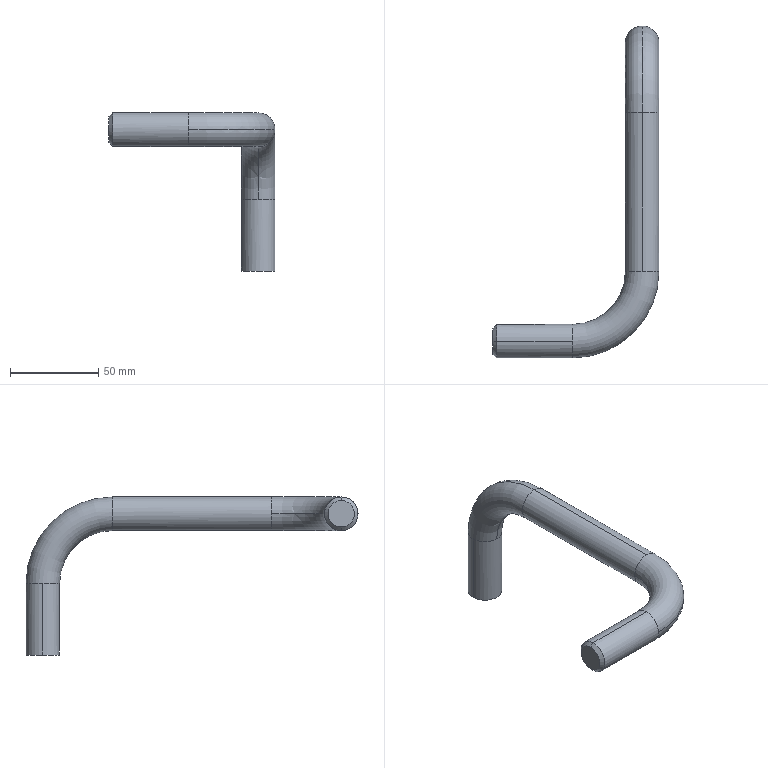Part | SolidWorks | features 3DProfileFeature 2, Chamfer 1, Sweep 1 | 1 solid | 14 faces | box 94 x 188 x 89.5 mm | volume 84832 mm3 | cylinder 6 | torus 4 | cone 2 | plane 2 | commonest cylinder face diameters 19 x6
STEP:
#1=CARTESIAN_POINT('',(9.5,-129.5,80.));
#2=VERTEX_POINT('',#1);
#3=CARTESIAN_POINT('',(0.,-129.5,70.5));
#4=VERTEX_POINT('',#3);
#5=CARTESIAN_POINT('',(0.,-129.5,80.));
#6=DIRECTION('',(0.,1.,0.));
#7=DIRECTION('',(0.,0.,-1.));
#8=AXIS2_PLACEMENT_3D('',#5,#6,#7);
#9=CIRCLE('',#8,9.5);
#10=EDGE_CURVE('',#2,#4,#9,.T.);
#11=ORIENTED_EDGE('',*,*,#10,.F.);
#12=CARTESIAN_POINT('',(-39.5,-178.5,80.));
#13=VERTEX_POINT('',#12);
#14=CARTESIAN_POINT('',(-39.5,-129.5,80.));
#15=DIRECTION('',(0.,0.,-1.));
#16=DIRECTION('',(-1.,0.,0.));
#17=AXIS2_PLACEMENT_3D('',#14,#15,#16);
#18=CIRCLE('',#17,49.);
#19=EDGE_CURVE('',#2,#13,#18,.T.);
#20=ORIENTED_EDGE('',*,*,#19,.T.);
#21=CARTESIAN_POINT('',(-39.5,-169.,70.5));
#22=VERTEX_POINT('',#21);
#23=CARTESIAN_POINT('',(-39.5,-169.,80.));
#24=DIRECTION('',(1.,0.,0.));
#25=DIRECTION('',(0.,0.,-1.));
#26=AXIS2_PLACEMENT_3D('',#23,#24,#25);
#27=CIRCLE('',#26,9.5);
#28=EDGE_CURVE('',#13,#22,#27,.T.);
#29=ORIENTED_EDGE('',*,*,#28,.T.);
#30=CARTESIAN_POINT('',(-39.5,-159.5,80.));
#31=VERTEX_POINT('',#30);
#32=CARTESIAN_POINT('',(-39.5,-169.,80.));
#33=DIRECTION('',(1.,0.,0.));
#34=DIRECTION('',(0.,0.,-1.));
#35=AXIS2_PLACEMENT_3D('',#32,#33,#34);
#36=CIRCLE('',#35,9.5);
#37=EDGE_CURVE('',#22,#31,#36,.T.);
#38=ORIENTED_EDGE('',*,*,#37,.T.);
#39=CARTESIAN_POINT('',(-9.5,-129.5,80.));
#40=VERTEX_POINT('',#39);
#41=CARTESIAN_POINT('',(-39.5,-129.5,80.));
#42=DIRECTION('',(0.,0.,-1.));
#43=DIRECTION('',(-1.,0.,0.));
#44=AXIS2_PLACEMENT_3D('',#41,#42,#43);
#45=CIRCLE('',#44,30.);
#46=EDGE_CURVE('',#40,#31,#45,.T.);
#47=ORIENTED_EDGE('',*,*,#46,.F.);
#48=CARTESIAN_POINT('',(0.,-129.5,80.));
#49=DIRECTION('',(0.,1.,0.));
#50=DIRECTION('',(0.,0.,-1.));
#51=AXIS2_PLACEMENT_3D('',#48,#49,#50);
#52=CIRCLE('',#51,9.5);
#53=EDGE_CURVE('',#4,#40,#52,.T.);
#54=ORIENTED_EDGE('',*,*,#53,.F.);
#55=EDGE_LOOP('',(#11,#20,#29,#38,#47,#54));
#56=FACE_OUTER_BOUND('',#55,.T.);
#57=CARTESIAN_POINT('',(-39.5,-129.5,80.));
#58=DIRECTION('',(0.,0.,-1.));
#59=DIRECTION('',(-1.,0.,0.));
#60=AXIS2_PLACEMENT_3D('',#57,#58,#59);
#61=TOROIDAL_SURFACE('',#60,39.5,9.5);
#62=ADVANCED_FACE('',(#56),#61,.T.);
#63=CARTESIAN_POINT('',(0.,9.5,40.5));
#64=VERTEX_POINT('',#63);
#65=CARTESIAN_POINT('',(9.5,0.,40.5));
#66=VERTEX_POINT('',#65);
#67=CARTESIAN_POINT('',(0.,0.,40.5));
#68=DIRECTION('',(0.,0.,-1.));
#69=DIRECTION('',(0.,-1.,0.));
#70=AXIS2_PLACEMENT_3D('',#67,#68,#69);
#71=CIRCLE('',#70,9.5);
#72=EDGE_CURVE('',#64,#66,#71,.T.);
#73=ORIENTED_EDGE('',*,*,#72,.F.);
#74=CARTESIAN_POINT('',(0.,-39.5,89.5));
#75=VERTEX_POINT('',#74);
#76=CARTESIAN_POINT('',(0.,-39.5,40.5));
#77=DIRECTION('',(1.,0.,0.));
#78=DIRECTION('',(0.,0.,-1.));
#79=AXIS2_PLACEMENT_3D('',#76,#77,#78);
#80=CIRCLE('',#79,49.);
#81=EDGE_CURVE('',#64,#75,#80,.T.);
#82=ORIENTED_EDGE('',*,*,#81,.T.);
#83=CARTESIAN_POINT('',(0.,-39.5,70.5));
#84=VERTEX_POINT('',#83);
#85=CARTESIAN_POINT('',(0.,-39.5,80.));
#86=DIRECTION('',(0.,1.,0.));
#87=DIRECTION('',(0.,0.,-1.));
#88=AXIS2_PLACEMENT_3D('',#85,#86,#87);
#89=CIRCLE('',#88,9.5);
#90=EDGE_CURVE('',#75,#84,#89,.T.);
#91=ORIENTED_EDGE('',*,*,#90,.T.);
#92=CARTESIAN_POINT('',(0.,-9.5,40.5));
#93=VERTEX_POINT('',#92);
#94=CARTESIAN_POINT('',(0.,-39.5,40.5));
#95=DIRECTION('',(1.,0.,0.));
#96=DIRECTION('',(0.,0.,-1.));
#97=AXIS2_PLACEMENT_3D('',#94,#95,#96);
#98=CIRCLE('',#97,30.);
#99=EDGE_CURVE('',#93,#84,#98,.T.);
#100=ORIENTED_EDGE('',*,*,#99,.F.);
#101=CARTESIAN_POINT('',(0.,0.,40.5));
#102=DIRECTION('',(0.,0.,-1.));
#103=DIRECTION('',(0.,-1.,0.));
#104=AXIS2_PLACEMENT_3D('',#101,#102,#103);
#105=CIRCLE('',#104,9.5);
#106=EDGE_CURVE('',#66,#93,#105,.T.);
#107=ORIENTED_EDGE('',*,*,#106,.F.);
#108=EDGE_LOOP('',(#73,#82,#91,#100,#107));
#109=FACE_OUTER_BOUND('',#108,.T.);
#110=CARTESIAN_POINT('',(0.,-39.5,40.5));
#111=DIRECTION('',(1.,0.,0.));
#112=DIRECTION('',(0.,0.,-1.));
#113=AXIS2_PLACEMENT_3D('',#110,#111,#112);
#114=TOROIDAL_SURFACE('',#113,39.5,9.5);
#115=ADVANCED_FACE('',(#109),#114,.T.);
#116=CARTESIAN_POINT('',(-84.5,-169.,87.5));
#117=VERTEX_POINT('',#116);
#118=CARTESIAN_POINT('',(-84.5,-169.,72.5));
#119=VERTEX_POINT('',#118);
#120=CARTESIAN_POINT('',(-84.5,-169.,80.));
#121=DIRECTION('',(-1.,0.,0.));
#122=DIRECTION('',(0.,0.,-1.));
#123=AXIS2_PLACEMENT_3D('',#120,#121,#122);
#124=CIRCLE('',#123,7.5);
#125=EDGE_CURVE('',#117,#119,#124,.T.);
#126=ORIENTED_EDGE('',*,*,#125,.F.);
#127=CARTESIAN_POINT('',(-82.5,-169.,89.5));
#128=VERTEX_POINT('',#127);
#129=CARTESIAN_POINT('',(-82.5,-169.,89.5));
#130=DIRECTION('',(0.7071,0.,0.7071));
#131=VECTOR('',#130,1000.);
#132=LINE('',#129,#131);
#133=EDGE_CURVE('',#117,#128,#132,.T.);
#134=ORIENTED_EDGE('',*,*,#133,.T.);
#135=CARTESIAN_POINT('',(-82.5,-169.,70.5));
#136=VERTEX_POINT('',#135);
#137=CARTESIAN_POINT('',(-82.5,-169.,80.));
#138=DIRECTION('',(1.,0.,0.));
#139=DIRECTION('',(0.,0.,-1.));
#140=AXIS2_PLACEMENT_3D('',#137,#138,#139);
#141=CIRCLE('',#140,9.5);
#142=EDGE_CURVE('',#136,#128,#141,.T.);
#143=ORIENTED_EDGE('',*,*,#142,.F.);
#144=CARTESIAN_POINT('',(-82.5,-169.,70.5));
#145=DIRECTION('',(0.7071,0.,-0.7071));
#146=VECTOR('',#145,1000.);
#147=LINE('',#144,#146);
#148=EDGE_CURVE('',#119,#136,#147,.T.);
#149=ORIENTED_EDGE('',*,*,#148,.F.);
#150=EDGE_LOOP('',(#126,#134,#143,#149));
#151=FACE_OUTER_BOUND('',#150,.T.);
#152=CARTESIAN_POINT('',(-82.5,-169.,80.));
#153=DIRECTION('',(1.,0.,0.));
#154=DIRECTION('',(0.,0.,-1.));
#155=AXIS2_PLACEMENT_3D('',#152,#153,#154);
#156=CONICAL_SURFACE('',#155,9.5,0.7854);
#157=ADVANCED_FACE('',(#151),#156,.T.);
#158=ORIENTED_EDGE('',*,*,#37,.F.);
#159=CARTESIAN_POINT('',(-39.5,-169.,70.5));
#160=DIRECTION('',(-1.,0.,0.));
#161=VECTOR('',#160,1000.);
#162=LINE('',#159,#161);
#163=EDGE_CURVE('',#22,#136,#162,.T.);
#164=ORIENTED_EDGE('',*,*,#163,.T.);
#165=ORIENTED_EDGE('',*,*,#142,.T.);
#166=CARTESIAN_POINT('',(-39.5,-169.,89.5));
#167=VERTEX_POINT('',#166);
#168=CARTESIAN_POINT('',(-39.5,-169.,89.5));
#169=DIRECTION('',(-1.,0.,0.));
#170=VECTOR('',#169,1000.);
#171=LINE('',#168,#170);
#172=EDGE_CURVE('',#167,#128,#171,.T.);
#173=ORIENTED_EDGE('',*,*,#172,.F.);
#174=CARTESIAN_POINT('',(-39.5,-169.,80.));
#175=DIRECTION('',(1.,0.,0.));
#176=DIRECTION('',(0.,0.,-1.));
#177=AXIS2_PLACEMENT_3D('',#174,#175,#176);
#178=CIRCLE('',#177,9.5);
#179=EDGE_CURVE('',#31,#167,#178,.T.);
#180=ORIENTED_EDGE('',*,*,#179,.F.);
#181=EDGE_LOOP('',(#158,#164,#165,#173,#180));
#182=FACE_OUTER_BOUND('',#181,.T.);
#183=CARTESIAN_POINT('',(-39.5,-169.,80.));
#184=DIRECTION('',(-1.,0.,0.));
#185=DIRECTION('',(0.,0.,1.));
#186=AXIS2_PLACEMENT_3D('',#183,#184,#185);
#187=CYLINDRICAL_SURFACE('',#186,9.5);
#188=ADVANCED_FACE('',(#182),#187,.T.);
#189=ORIENTED_EDGE('',*,*,#90,.F.);
#190=CARTESIAN_POINT('',(0.,-129.5,89.5));
#191=VERTEX_POINT('',#190);
#192=CARTESIAN_POINT('',(0.,-39.5,89.5));
#193=DIRECTION('',(0.,-1.,0.));
#194=VECTOR('',#193,1000.);
#195=LINE('',#192,#194);
#196=EDGE_CURVE('',#75,#191,#195,.T.);
#197=ORIENTED_EDGE('',*,*,#196,.T.);
#198=CARTESIAN_POINT('',(0.,-129.5,80.));
#199=DIRECTION('',(0.,1.,0.));
#200=DIRECTION('',(0.,0.,-1.));
#201=AXIS2_PLACEMENT_3D('',#198,#199,#200);
#202=CIRCLE('',#201,9.5);
#203=EDGE_CURVE('',#191,#2,#202,.T.);
#204=ORIENTED_EDGE('',*,*,#203,.T.);
#205=ORIENTED_EDGE('',*,*,#10,.T.);
#206=CARTESIAN_POINT('',(0.,-39.5,70.5));
#207=DIRECTION('',(0.,-1.,0.));
#208=VECTOR('',#207,1000.);
#209=LINE('',#206,#208);
#210=EDGE_CURVE('',#84,#4,#209,.T.);
#211=ORIENTED_EDGE('',*,*,#210,.F.);
#212=EDGE_LOOP('',(#189,#197,#204,#205,#211));
#213=FACE_OUTER_BOUND('',#212,.T.);
#214=CARTESIAN_POINT('',(0.,-39.5,80.));
#215=DIRECTION('',(0.,-1.,0.));
#216=DIRECTION('',(0.,0.,-1.));
#217=AXIS2_PLACEMENT_3D('',#214,#215,#216);
#218=CYLINDRICAL_SURFACE('',#217,9.5);
#219=ADVANCED_FACE('',(#213),#218,.T.);
#220=CARTESIAN_POINT('',(-9.5,0.,0.));
#221=VERTEX_POINT('',#220);
#222=CARTESIAN_POINT('',(9.5,0.,0.));
#223=VERTEX_POINT('',#222);
#224=CARTESIAN_POINT('',(0.,0.,0.));
#225=DIRECTION('',(0.,0.,-1.));
#226=DIRECTION('',(0.,-1.,0.));
#227=AXIS2_PLACEMENT_3D('',#224,#225,#226);
#228=CIRCLE('',#227,9.5);
#229=EDGE_CURVE('',#221,#223,#228,.T.);
#230=ORIENTED_EDGE('',*,*,#229,.F.);
#231=CARTESIAN_POINT('',(-9.5,0.,40.5));
#232=VERTEX_POINT('',#231);
#233=CARTESIAN_POINT('',(-9.5,0.,0.));
#234=DIRECTION('',(0.,0.,1.));
#235=VECTOR('',#234,1000.);
#236=LINE('',#233,#235);
#237=EDGE_CURVE('',#221,#232,#236,.T.);
#238=ORIENTED_EDGE('',*,*,#237,.T.);
#239=CARTESIAN_POINT('',(0.,0.,40.5));
#240=DIRECTION('',(0.,0.,-1.));
#241=DIRECTION('',(0.,-1.,0.));
#242=AXIS2_PLACEMENT_3D('',#239,#240,#241);
#243=CIRCLE('',#242,9.5);
#244=EDGE_CURVE('',#232,#64,#243,.T.);
#245=ORIENTED_EDGE('',*,*,#244,.T.);
#246=ORIENTED_EDGE('',*,*,#72,.T.);
#247=CARTESIAN_POINT('',(9.5,0.,0.));
#248=DIRECTION('',(0.,0.,1.));
#249=VECTOR('',#248,1000.);
#250=LINE('',#247,#249);
#251=EDGE_CURVE('',#223,#66,#250,.T.);
#252=ORIENTED_EDGE('',*,*,#251,.F.);
#253=EDGE_LOOP('',(#230,#238,#245,#246,#252));
#254=FACE_OUTER_BOUND('',#253,.T.);
#255=CARTESIAN_POINT('',(0.,0.,0.));
#256=DIRECTION('',(0.,0.,1.));
#257=DIRECTION('',(1.,0.,0.));
#258=AXIS2_PLACEMENT_3D('',#255,#256,#257);
#259=CYLINDRICAL_SURFACE('',#258,9.5);
#260=ADVANCED_FACE('',(#254),#259,.T.);
#261=ORIENTED_EDGE('',*,*,#163,.F.);
#262=ORIENTED_EDGE('',*,*,#28,.F.);
#263=CARTESIAN_POINT('',(-39.5,-169.,80.));
#264=DIRECTION('',(1.,0.,0.));
#265=DIRECTION('',(0.,0.,-1.));
#266=AXIS2_PLACEMENT_3D('',#263,#264,#265);
#267=CIRCLE('',#266,9.5);
#268=EDGE_CURVE('',#167,#13,#267,.T.);
#269=ORIENTED_EDGE('',*,*,#268,.F.);
#270=ORIENTED_EDGE('',*,*,#172,.T.);
#271=CARTESIAN_POINT('',(-82.5,-169.,80.));
#272=DIRECTION('',(1.,0.,0.));
#273=DIRECTION('',(0.,0.,-1.));
#274=AXIS2_PLACEMENT_3D('',#271,#272,#273);
#275=CIRCLE('',#274,9.5);
#276=EDGE_CURVE('',#128,#136,#275,.T.);
#277=ORIENTED_EDGE('',*,*,#276,.T.);
#278=EDGE_LOOP('',(#261,#262,#269,#270,#277));
#279=FACE_OUTER_BOUND('',#278,.T.);
#280=CARTESIAN_POINT('',(-39.5,-169.,80.));
#281=DIRECTION('',(-1.,0.,0.));
#282=DIRECTION('',(0.,0.,1.));
#283=AXIS2_PLACEMENT_3D('',#280,#281,#282);
#284=CYLINDRICAL_SURFACE('',#283,9.5);
#285=ADVANCED_FACE('',(#279),#284,.T.);
#286=ORIENTED_EDGE('',*,*,#19,.F.);
#287=ORIENTED_EDGE('',*,*,#203,.F.);
#288=CARTESIAN_POINT('',(0.,-129.5,80.));
#289=DIRECTION('',(0.,1.,0.));
#290=DIRECTION('',(0.,0.,-1.));
#291=AXIS2_PLACEMENT_3D('',#288,#289,#290);
#292=CIRCLE('',#291,9.5);
#293=EDGE_CURVE('',#40,#191,#292,.T.);
#294=ORIENTED_EDGE('',*,*,#293,.F.);
#295=ORIENTED_EDGE('',*,*,#46,.T.);
#296=ORIENTED_EDGE('',*,*,#179,.T.);
#297=ORIENTED_EDGE('',*,*,#268,.T.);
#298=EDGE_LOOP('',(#286,#287,#294,#295,#296,#297));
#299=FACE_OUTER_BOUND('',#298,.T.);
#300=CARTESIAN_POINT('',(-39.5,-129.5,80.));
#301=DIRECTION('',(0.,0.,-1.));
#302=DIRECTION('',(-1.,0.,0.));
#303=AXIS2_PLACEMENT_3D('',#300,#301,#302);
#304=TOROIDAL_SURFACE('',#303,39.5,9.5);
#305=ADVANCED_FACE('',(#299),#304,.T.);
#306=ORIENTED_EDGE('',*,*,#196,.F.);
#307=CARTESIAN_POINT('',(0.,-39.5,80.));
#308=DIRECTION('',(0.,1.,0.));
#309=DIRECTION('',(0.,0.,-1.));
#310=AXIS2_PLACEMENT_3D('',#307,#308,#309);
#311=CIRCLE('',#310,9.5);
#312=EDGE_CURVE('',#84,#75,#311,.T.);
#313=ORIENTED_EDGE('',*,*,#312,.F.);
#314=ORIENTED_EDGE('',*,*,#210,.T.);
#315=ORIENTED_EDGE('',*,*,#53,.T.);
#316=ORIENTED_EDGE('',*,*,#293,.T.);
#317=EDGE_LOOP('',(#306,#313,#314,#315,#316));
#318=FACE_OUTER_BOUND('',#317,.T.);
#319=CARTESIAN_POINT('',(0.,-39.5,80.));
#320=DIRECTION('',(0.,-1.,0.));
#321=DIRECTION('',(0.,0.,-1.));
#322=AXIS2_PLACEMENT_3D('',#319,#320,#321);
#323=CYLINDRICAL_SURFACE('',#322,9.5);
#324=ADVANCED_FACE('',(#318),#323,.T.);
#325=ORIENTED_EDGE('',*,*,#81,.F.);
#326=ORIENTED_EDGE('',*,*,#244,.F.);
#327=CARTESIAN_POINT('',(0.,0.,40.5));
#328=DIRECTION('',(0.,0.,-1.));
#329=DIRECTION('',(0.,-1.,0.));
#330=AXIS2_PLACEMENT_3D('',#327,#328,#329);
#331=CIRCLE('',#330,9.5);
#332=EDGE_CURVE('',#93,#232,#331,.T.);
#333=ORIENTED_EDGE('',*,*,#332,.F.);
#334=ORIENTED_EDGE('',*,*,#99,.T.);
#335=ORIENTED_EDGE('',*,*,#312,.T.);
#336=EDGE_LOOP('',(#325,#326,#333,#334,#335));
#337=FACE_OUTER_BOUND('',#336,.T.);
#338=CARTESIAN_POINT('',(0.,-39.5,40.5));
#339=DIRECTION('',(1.,0.,0.));
#340=DIRECTION('',(0.,0.,-1.));
#341=AXIS2_PLACEMENT_3D('',#338,#339,#340);
#342=TOROIDAL_SURFACE('',#341,39.5,9.5);
#343=ADVANCED_FACE('',(#337),#342,.T.);
#344=ORIENTED_EDGE('',*,*,#237,.F.);
#345=CARTESIAN_POINT('',(0.,0.,0.));
#346=DIRECTION('',(0.,0.,-1.));
#347=DIRECTION('',(0.,-1.,0.));
#348=AXIS2_PLACEMENT_3D('',#345,#346,#347);
#349=CIRCLE('',#348,9.5);
#350=EDGE_CURVE('',#223,#221,#349,.T.);
#351=ORIENTED_EDGE('',*,*,#350,.F.);
#352=ORIENTED_EDGE('',*,*,#251,.T.);
#353=ORIENTED_EDGE('',*,*,#106,.T.);
#354=ORIENTED_EDGE('',*,*,#332,.T.);
#355=EDGE_LOOP('',(#344,#351,#352,#353,#354));
#356=FACE_OUTER_BOUND('',#355,.T.);
#357=CARTESIAN_POINT('',(0.,0.,0.));
#358=DIRECTION('',(0.,0.,1.));
#359=DIRECTION('',(1.,0.,0.));
#360=AXIS2_PLACEMENT_3D('',#357,#358,#359);
#361=CYLINDRICAL_SURFACE('',#360,9.5);
#362=ADVANCED_FACE('',(#356),#361,.T.);
#363=CARTESIAN_POINT('',(-84.5,-169.,80.));
#364=DIRECTION('',(-1.,0.,0.));
#365=DIRECTION('',(0.,0.,-1.));
#366=AXIS2_PLACEMENT_3D('',#363,#364,#365);
#367=CIRCLE('',#366,7.5);
#368=EDGE_CURVE('',#119,#117,#367,.T.);
#369=ORIENTED_EDGE('',*,*,#368,.T.);
#370=ORIENTED_EDGE('',*,*,#125,.T.);
#371=EDGE_LOOP('',(#369,#370));
#372=FACE_OUTER_BOUND('',#371,.T.);
#373=CARTESIAN_POINT('',(-84.5,-169.,80.));
#374=DIRECTION('',(1.,0.,0.));
#375=DIRECTION('',(0.,0.,-1.));
#376=AXIS2_PLACEMENT_3D('',#373,#374,#375);
#377=PLANE('',#376);
#378=ADVANCED_FACE('',(#372),#377,.F.);
#379=ORIENTED_EDGE('',*,*,#350,.T.);
#380=ORIENTED_EDGE('',*,*,#229,.T.);
#381=EDGE_LOOP('',(#379,#380));
#382=FACE_OUTER_BOUND('',#381,.T.);
#383=CARTESIAN_POINT('',(0.,0.,0.));
#384=DIRECTION('',(0.,0.,-1.));
#385=DIRECTION('',(0.,-1.,0.));
#386=AXIS2_PLACEMENT_3D('',#383,#384,#385);
#387=PLANE('',#386);
#388=ADVANCED_FACE('',(#382),#387,.T.);
#389=ORIENTED_EDGE('',*,*,#133,.F.);
#390=ORIENTED_EDGE('',*,*,#368,.F.);
#391=ORIENTED_EDGE('',*,*,#148,.T.);
#392=ORIENTED_EDGE('',*,*,#276,.F.);
#393=EDGE_LOOP('',(#389,#390,#391,#392));
#394=FACE_OUTER_BOUND('',#393,.T.);
#395=CARTESIAN_POINT('',(-82.5,-169.,80.));
#396=DIRECTION('',(1.,0.,0.));
#397=DIRECTION('',(0.,0.,-1.));
#398=AXIS2_PLACEMENT_3D('',#395,#396,#397);
#399=CONICAL_SURFACE('',#398,9.5,0.7854);
#400=ADVANCED_FACE('',(#394),#399,.T.);
#401=CLOSED_SHELL('',(#62,#115,#157,#188,#219,#260,#285,#305,#324,#343,#362,#378,#388,#400));
#402=MANIFOLD_SOLID_BREP('',#401);
#403=CARTESIAN_POINT('',(0.,0.,0.));
#404=DIRECTION('',(0.,0.,1.));
#405=DIRECTION('',(1.,0.,0.));
#406=AXIS2_PLACEMENT_3D('',#403,#404,#405);
#407=(LENGTH_UNIT()NAMED_UNIT(*)SI_UNIT(.MILLI.,.METRE.));
#408=UNCERTAINTY_MEASURE_WITH_UNIT(LENGTH_MEASURE(0.00001),#407,'','');
#409=(NAMED_UNIT(*)PLANE_ANGLE_UNIT()SI_UNIT($,.RADIAN.));
#410=(NAMED_UNIT(*)SI_UNIT($,.STERADIAN.)SOLID_ANGLE_UNIT());
#411=(GEOMETRIC_REPRESENTATION_CONTEXT(3)GLOBAL_UNCERTAINTY_ASSIGNED_CONTEXT((#408))GLOBAL_UNIT_ASSIGNED_CONTEXT((#407,#409,#410))REPRESENTATION_CONTEXT('',''));
#412=ADVANCED_BREP_SHAPE_REPRESENTATION('',(#402,#406),#411);